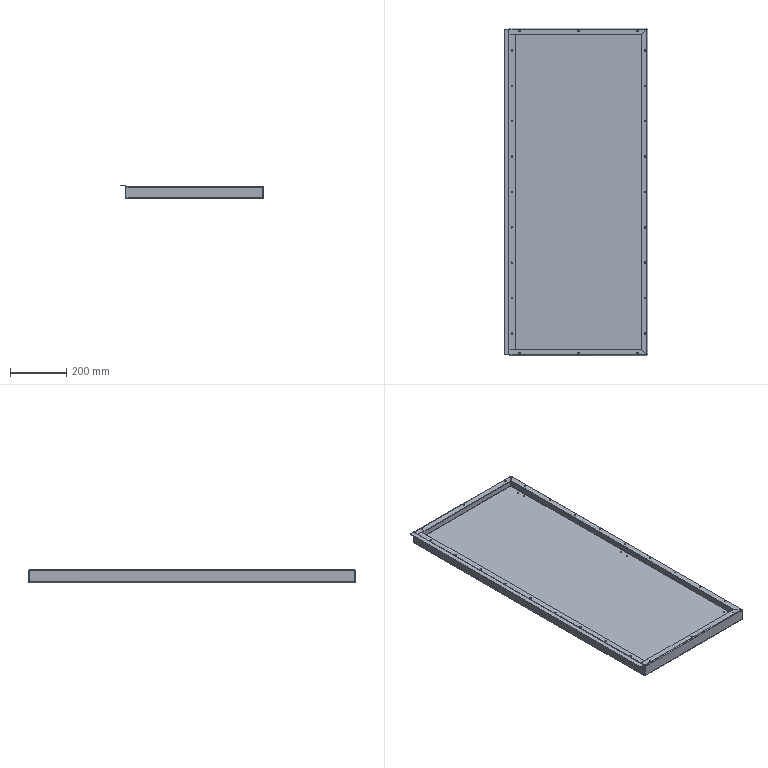Part | SolidWorks | 2 solids | 136 faces | box 512 x 1168 x 48 mm | volume 1999413 mm3 | cylinder 76 | plane 48 | spline 12 | commonest cylinder face diameters 5 x60 1.473 x8 6.473 x8